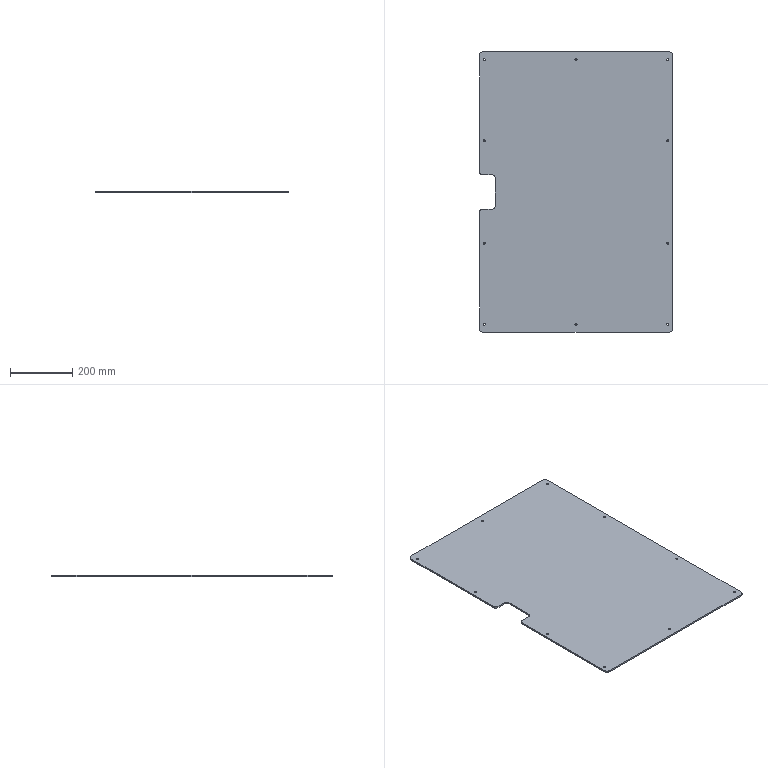Part | STEP file | 11-FG-00911 | 1 solid | 38 faces | box 618 x 900 x 5 mm | volume 2751412 mm3 | cylinder 28 | plane 10 | commonest cylinder face diameters 6.5 x20 20 x8
STEP:
#1=CARTESIAN_POINT('',(-3.25,424.,0.));
#2=VERTEX_POINT('',#1);
#3=CARTESIAN_POINT('',(3.25,424.,0.));
#4=VERTEX_POINT('',#3);
#5=CARTESIAN_POINT('',(0.,424.,0.));
#6=DIRECTION('',(0.,0.,1.));
#7=DIRECTION('',(1.,0.,0.));
#8=AXIS2_PLACEMENT_3D('',#5,#6,#7);
#9=CIRCLE('',#8,3.25);
#10=EDGE_CURVE('',#2,#4,#9,.T.);
#11=ORIENTED_EDGE('',*,*,#10,.F.);
#12=CARTESIAN_POINT('',(-3.25,424.,5.));
#13=VERTEX_POINT('',#12);
#14=CARTESIAN_POINT('',(-3.25,424.,-5.));
#15=DIRECTION('',(0.,0.,1.));
#16=VECTOR('',#15,1000.);
#17=LINE('',#14,#16);
#18=EDGE_CURVE('',#2,#13,#17,.T.);
#19=ORIENTED_EDGE('',*,*,#18,.T.);
#20=CARTESIAN_POINT('',(3.25,424.,5.));
#21=VERTEX_POINT('',#20);
#22=CARTESIAN_POINT('',(0.,424.,5.));
#23=DIRECTION('',(0.,0.,1.));
#24=DIRECTION('',(1.,0.,0.));
#25=AXIS2_PLACEMENT_3D('',#22,#23,#24);
#26=CIRCLE('',#25,3.25);
#27=EDGE_CURVE('',#13,#21,#26,.T.);
#28=ORIENTED_EDGE('',*,*,#27,.T.);
#29=CARTESIAN_POINT('',(3.25,424.,-5.));
#30=DIRECTION('',(0.,0.,1.));
#31=VECTOR('',#30,1000.);
#32=LINE('',#29,#31);
#33=EDGE_CURVE('',#4,#21,#32,.T.);
#34=ORIENTED_EDGE('',*,*,#33,.F.);
#35=EDGE_LOOP('',(#11,#19,#28,#34));
#36=FACE_OUTER_BOUND('',#35,.T.);
#37=CARTESIAN_POINT('',(0.,424.,-5.));
#38=DIRECTION('',(0.,0.,1.));
#39=DIRECTION('',(1.,0.,0.));
#40=AXIS2_PLACEMENT_3D('',#37,#38,#39);
#41=CYLINDRICAL_SURFACE('',#40,3.25);
#42=ADVANCED_FACE('',(#36),#41,.F.);
#43=CARTESIAN_POINT('',(-297.25,424.,0.));
#44=VERTEX_POINT('',#43);
#45=CARTESIAN_POINT('',(-290.75,424.,0.));
#46=VERTEX_POINT('',#45);
#47=CARTESIAN_POINT('',(-294.,424.,0.));
#48=DIRECTION('',(0.,0.,1.));
#49=DIRECTION('',(1.,0.,0.));
#50=AXIS2_PLACEMENT_3D('',#47,#48,#49);
#51=CIRCLE('',#50,3.25);
#52=EDGE_CURVE('',#44,#46,#51,.T.);
#53=ORIENTED_EDGE('',*,*,#52,.F.);
#54=CARTESIAN_POINT('',(-297.25,424.,5.));
#55=VERTEX_POINT('',#54);
#56=CARTESIAN_POINT('',(-297.25,424.,-5.));
#57=DIRECTION('',(0.,0.,1.));
#58=VECTOR('',#57,1000.);
#59=LINE('',#56,#58);
#60=EDGE_CURVE('',#44,#55,#59,.T.);
#61=ORIENTED_EDGE('',*,*,#60,.T.);
#62=CARTESIAN_POINT('',(-290.75,424.,5.));
#63=VERTEX_POINT('',#62);
#64=CARTESIAN_POINT('',(-294.,424.,5.));
#65=DIRECTION('',(0.,0.,1.));
#66=DIRECTION('',(1.,0.,0.));
#67=AXIS2_PLACEMENT_3D('',#64,#65,#66);
#68=CIRCLE('',#67,3.25);
#69=EDGE_CURVE('',#55,#63,#68,.T.);
#70=ORIENTED_EDGE('',*,*,#69,.T.);
#71=CARTESIAN_POINT('',(-290.75,424.,-5.));
#72=DIRECTION('',(0.,0.,1.));
#73=VECTOR('',#72,1000.);
#74=LINE('',#71,#73);
#75=EDGE_CURVE('',#46,#63,#74,.T.);
#76=ORIENTED_EDGE('',*,*,#75,.F.);
#77=EDGE_LOOP('',(#53,#61,#70,#76));
#78=FACE_OUTER_BOUND('',#77,.T.);
#79=CARTESIAN_POINT('',(-294.,424.,-5.));
#80=DIRECTION('',(0.,0.,1.));
#81=DIRECTION('',(1.,0.,0.));
#82=AXIS2_PLACEMENT_3D('',#79,#80,#81);
#83=CYLINDRICAL_SURFACE('',#82,3.25);
#84=ADVANCED_FACE('',(#78),#83,.F.);
#85=CARTESIAN_POINT('',(-297.25,164.,0.));
#86=VERTEX_POINT('',#85);
#87=CARTESIAN_POINT('',(-290.75,164.,0.));
#88=VERTEX_POINT('',#87);
#89=CARTESIAN_POINT('',(-294.,164.,0.));
#90=DIRECTION('',(0.,0.,1.));
#91=DIRECTION('',(1.,0.,0.));
#92=AXIS2_PLACEMENT_3D('',#89,#90,#91);
#93=CIRCLE('',#92,3.25);
#94=EDGE_CURVE('',#86,#88,#93,.T.);
#95=ORIENTED_EDGE('',*,*,#94,.F.);
#96=CARTESIAN_POINT('',(-297.25,164.,5.));
#97=VERTEX_POINT('',#96);
#98=CARTESIAN_POINT('',(-297.25,164.,-5.));
#99=DIRECTION('',(0.,0.,1.));
#100=VECTOR('',#99,1000.);
#101=LINE('',#98,#100);
#102=EDGE_CURVE('',#86,#97,#101,.T.);
#103=ORIENTED_EDGE('',*,*,#102,.T.);
#104=CARTESIAN_POINT('',(-290.75,164.,5.));
#105=VERTEX_POINT('',#104);
#106=CARTESIAN_POINT('',(-294.,164.,5.));
#107=DIRECTION('',(0.,0.,1.));
#108=DIRECTION('',(1.,0.,0.));
#109=AXIS2_PLACEMENT_3D('',#106,#107,#108);
#110=CIRCLE('',#109,3.25);
#111=EDGE_CURVE('',#97,#105,#110,.T.);
#112=ORIENTED_EDGE('',*,*,#111,.T.);
#113=CARTESIAN_POINT('',(-290.75,164.,-5.));
#114=DIRECTION('',(0.,0.,1.));
#115=VECTOR('',#114,1000.);
#116=LINE('',#113,#115);
#117=EDGE_CURVE('',#88,#105,#116,.T.);
#118=ORIENTED_EDGE('',*,*,#117,.F.);
#119=EDGE_LOOP('',(#95,#103,#112,#118));
#120=FACE_OUTER_BOUND('',#119,.T.);
#121=CARTESIAN_POINT('',(-294.,164.,-5.));
#122=DIRECTION('',(0.,0.,1.));
#123=DIRECTION('',(1.,0.,0.));
#124=AXIS2_PLACEMENT_3D('',#121,#122,#123);
#125=CYLINDRICAL_SURFACE('',#124,3.25);
#126=ADVANCED_FACE('',(#120),#125,.F.);
#127=CARTESIAN_POINT('',(-297.25,-164.,0.));
#128=VERTEX_POINT('',#127);
#129=CARTESIAN_POINT('',(-290.75,-164.,0.));
#130=VERTEX_POINT('',#129);
#131=CARTESIAN_POINT('',(-294.,-164.,0.));
#132=DIRECTION('',(0.,0.,1.));
#133=DIRECTION('',(1.,0.,0.));
#134=AXIS2_PLACEMENT_3D('',#131,#132,#133);
#135=CIRCLE('',#134,3.25);
#136=EDGE_CURVE('',#128,#130,#135,.T.);
#137=ORIENTED_EDGE('',*,*,#136,.F.);
#138=CARTESIAN_POINT('',(-297.25,-164.,5.));
#139=VERTEX_POINT('',#138);
#140=CARTESIAN_POINT('',(-297.25,-164.,-5.));
#141=DIRECTION('',(0.,0.,1.));
#142=VECTOR('',#141,1000.);
#143=LINE('',#140,#142);
#144=EDGE_CURVE('',#128,#139,#143,.T.);
#145=ORIENTED_EDGE('',*,*,#144,.T.);
#146=CARTESIAN_POINT('',(-290.75,-164.,5.));
#147=VERTEX_POINT('',#146);
#148=CARTESIAN_POINT('',(-294.,-164.,5.));
#149=DIRECTION('',(0.,0.,1.));
#150=DIRECTION('',(1.,0.,0.));
#151=AXIS2_PLACEMENT_3D('',#148,#149,#150);
#152=CIRCLE('',#151,3.25);
#153=EDGE_CURVE('',#139,#147,#152,.T.);
#154=ORIENTED_EDGE('',*,*,#153,.T.);
#155=CARTESIAN_POINT('',(-290.75,-164.,-5.));
#156=DIRECTION('',(0.,0.,1.));
#157=VECTOR('',#156,1000.);
#158=LINE('',#155,#157);
#159=EDGE_CURVE('',#130,#147,#158,.T.);
#160=ORIENTED_EDGE('',*,*,#159,.F.);
#161=EDGE_LOOP('',(#137,#145,#154,#160));
#162=FACE_OUTER_BOUND('',#161,.T.);
#163=CARTESIAN_POINT('',(-294.,-164.,-5.));
#164=DIRECTION('',(0.,0.,1.));
#165=DIRECTION('',(1.,0.,0.));
#166=AXIS2_PLACEMENT_3D('',#163,#164,#165);
#167=CYLINDRICAL_SURFACE('',#166,3.25);
#168=ADVANCED_FACE('',(#162),#167,.F.);
#169=CARTESIAN_POINT('',(-297.25,-424.,0.));
#170=VERTEX_POINT('',#169);
#171=CARTESIAN_POINT('',(-290.75,-424.,0.));
#172=VERTEX_POINT('',#171);
#173=CARTESIAN_POINT('',(-294.,-424.,0.));
#174=DIRECTION('',(0.,0.,1.));
#175=DIRECTION('',(1.,0.,0.));
#176=AXIS2_PLACEMENT_3D('',#173,#174,#175);
#177=CIRCLE('',#176,3.25);
#178=EDGE_CURVE('',#170,#172,#177,.T.);
#179=ORIENTED_EDGE('',*,*,#178,.F.);
#180=CARTESIAN_POINT('',(-297.25,-424.,5.));
#181=VERTEX_POINT('',#180);
#182=CARTESIAN_POINT('',(-297.25,-424.,-5.));
#183=DIRECTION('',(0.,0.,1.));
#184=VECTOR('',#183,1000.);
#185=LINE('',#182,#184);
#186=EDGE_CURVE('',#170,#181,#185,.T.);
#187=ORIENTED_EDGE('',*,*,#186,.T.);
#188=CARTESIAN_POINT('',(-290.75,-424.,5.));
#189=VERTEX_POINT('',#188);
#190=CARTESIAN_POINT('',(-294.,-424.,5.));
#191=DIRECTION('',(0.,0.,1.));
#192=DIRECTION('',(1.,0.,0.));
#193=AXIS2_PLACEMENT_3D('',#190,#191,#192);
#194=CIRCLE('',#193,3.25);
#195=EDGE_CURVE('',#181,#189,#194,.T.);
#196=ORIENTED_EDGE('',*,*,#195,.T.);
#197=CARTESIAN_POINT('',(-290.75,-424.,-5.));
#198=DIRECTION('',(0.,0.,1.));
#199=VECTOR('',#198,1000.);
#200=LINE('',#197,#199);
#201=EDGE_CURVE('',#172,#189,#200,.T.);
#202=ORIENTED_EDGE('',*,*,#201,.F.);
#203=EDGE_LOOP('',(#179,#187,#196,#202));
#204=FACE_OUTER_BOUND('',#203,.T.);
#205=CARTESIAN_POINT('',(-294.,-424.,-5.));
#206=DIRECTION('',(0.,0.,1.));
#207=DIRECTION('',(1.,0.,0.));
#208=AXIS2_PLACEMENT_3D('',#205,#206,#207);
#209=CYLINDRICAL_SURFACE('',#208,3.25);
#210=ADVANCED_FACE('',(#204),#209,.F.);
#211=CARTESIAN_POINT('',(-3.25,-424.,0.));
#212=VERTEX_POINT('',#211);
#213=CARTESIAN_POINT('',(3.25,-424.,0.));
#214=VERTEX_POINT('',#213);
#215=CARTESIAN_POINT('',(0.,-424.,0.));
#216=DIRECTION('',(0.,0.,1.));
#217=DIRECTION('',(1.,0.,0.));
#218=AXIS2_PLACEMENT_3D('',#215,#216,#217);
#219=CIRCLE('',#218,3.25);
#220=EDGE_CURVE('',#212,#214,#219,.T.);
#221=ORIENTED_EDGE('',*,*,#220,.F.);
#222=CARTESIAN_POINT('',(-3.25,-424.,5.));
#223=VERTEX_POINT('',#222);
#224=CARTESIAN_POINT('',(-3.25,-424.,-5.));
#225=DIRECTION('',(0.,0.,1.));
#226=VECTOR('',#225,1000.);
#227=LINE('',#224,#226);
#228=EDGE_CURVE('',#212,#223,#227,.T.);
#229=ORIENTED_EDGE('',*,*,#228,.T.);
#230=CARTESIAN_POINT('',(3.25,-424.,5.));
#231=VERTEX_POINT('',#230);
#232=CARTESIAN_POINT('',(0.,-424.,5.));
#233=DIRECTION('',(0.,0.,1.));
#234=DIRECTION('',(1.,0.,0.));
#235=AXIS2_PLACEMENT_3D('',#232,#233,#234);
#236=CIRCLE('',#235,3.25);
#237=EDGE_CURVE('',#223,#231,#236,.T.);
#238=ORIENTED_EDGE('',*,*,#237,.T.);
#239=CARTESIAN_POINT('',(3.25,-424.,-5.));
#240=DIRECTION('',(0.,0.,1.));
#241=VECTOR('',#240,1000.);
#242=LINE('',#239,#241);
#243=EDGE_CURVE('',#214,#231,#242,.T.);
#244=ORIENTED_EDGE('',*,*,#243,.F.);
#245=EDGE_LOOP('',(#221,#229,#238,#244));
#246=FACE_OUTER_BOUND('',#245,.T.);
#247=CARTESIAN_POINT('',(0.,-424.,-5.));
#248=DIRECTION('',(0.,0.,1.));
#249=DIRECTION('',(1.,0.,0.));
#250=AXIS2_PLACEMENT_3D('',#247,#248,#249);
#251=CYLINDRICAL_SURFACE('',#250,3.25);
#252=ADVANCED_FACE('',(#246),#251,.F.);
#253=CARTESIAN_POINT('',(290.75,-424.,0.));
#254=VERTEX_POINT('',#253);
#255=CARTESIAN_POINT('',(297.25,-424.,0.));
#256=VERTEX_POINT('',#255);
#257=CARTESIAN_POINT('',(294.,-424.,0.));
#258=DIRECTION('',(0.,0.,1.));
#259=DIRECTION('',(1.,0.,0.));
#260=AXIS2_PLACEMENT_3D('',#257,#258,#259);
#261=CIRCLE('',#260,3.25);
#262=EDGE_CURVE('',#254,#256,#261,.T.);
#263=ORIENTED_EDGE('',*,*,#262,.F.);
#264=CARTESIAN_POINT('',(290.75,-424.,5.));
#265=VERTEX_POINT('',#264);
#266=CARTESIAN_POINT('',(290.75,-424.,-5.));
#267=DIRECTION('',(0.,0.,1.));
#268=VECTOR('',#267,1000.);
#269=LINE('',#266,#268);
#270=EDGE_CURVE('',#254,#265,#269,.T.);
#271=ORIENTED_EDGE('',*,*,#270,.T.);
#272=CARTESIAN_POINT('',(297.25,-424.,5.));
#273=VERTEX_POINT('',#272);
#274=CARTESIAN_POINT('',(294.,-424.,5.));
#275=DIRECTION('',(0.,0.,1.));
#276=DIRECTION('',(1.,0.,0.));
#277=AXIS2_PLACEMENT_3D('',#274,#275,#276);
#278=CIRCLE('',#277,3.25);
#279=EDGE_CURVE('',#265,#273,#278,.T.);
#280=ORIENTED_EDGE('',*,*,#279,.T.);
#281=CARTESIAN_POINT('',(297.25,-424.,-5.));
#282=DIRECTION('',(0.,0.,1.));
#283=VECTOR('',#282,1000.);
#284=LINE('',#281,#283);
#285=EDGE_CURVE('',#256,#273,#284,.T.);
#286=ORIENTED_EDGE('',*,*,#285,.F.);
#287=EDGE_LOOP('',(#263,#271,#280,#286));
#288=FACE_OUTER_BOUND('',#287,.T.);
#289=CARTESIAN_POINT('',(294.,-424.,-5.));
#290=DIRECTION('',(0.,0.,1.));
#291=DIRECTION('',(1.,0.,0.));
#292=AXIS2_PLACEMENT_3D('',#289,#290,#291);
#293=CYLINDRICAL_SURFACE('',#292,3.25);
#294=ADVANCED_FACE('',(#288),#293,.F.);
#295=CARTESIAN_POINT('',(290.75,-164.,0.));
#296=VERTEX_POINT('',#295);
#297=CARTESIAN_POINT('',(297.25,-164.,0.));
#298=VERTEX_POINT('',#297);
#299=CARTESIAN_POINT('',(294.,-164.,0.));
#300=DIRECTION('',(0.,0.,1.));
#301=DIRECTION('',(1.,0.,0.));
#302=AXIS2_PLACEMENT_3D('',#299,#300,#301);
#303=CIRCLE('',#302,3.25);
#304=EDGE_CURVE('',#296,#298,#303,.T.);
#305=ORIENTED_EDGE('',*,*,#304,.F.);
#306=CARTESIAN_POINT('',(290.75,-164.,5.));
#307=VERTEX_POINT('',#306);
#308=CARTESIAN_POINT('',(290.75,-164.,-5.));
#309=DIRECTION('',(0.,0.,1.));
#310=VECTOR('',#309,1000.);
#311=LINE('',#308,#310);
#312=EDGE_CURVE('',#296,#307,#311,.T.);
#313=ORIENTED_EDGE('',*,*,#312,.T.);
#314=CARTESIAN_POINT('',(297.25,-164.,5.));
#315=VERTEX_POINT('',#314);
#316=CARTESIAN_POINT('',(294.,-164.,5.));
#317=DIRECTION('',(0.,0.,1.));
#318=DIRECTION('',(1.,0.,0.));
#319=AXIS2_PLACEMENT_3D('',#316,#317,#318);
#320=CIRCLE('',#319,3.25);
#321=EDGE_CURVE('',#307,#315,#320,.T.);
#322=ORIENTED_EDGE('',*,*,#321,.T.);
#323=CARTESIAN_POINT('',(297.25,-164.,-5.));
#324=DIRECTION('',(0.,0.,1.));
#325=VECTOR('',#324,1000.);
#326=LINE('',#323,#325);
#327=EDGE_CURVE('',#298,#315,#326,.T.);
#328=ORIENTED_EDGE('',*,*,#327,.F.);
#329=EDGE_LOOP('',(#305,#313,#322,#328));
#330=FACE_OUTER_BOUND('',#329,.T.);
#331=CARTESIAN_POINT('',(294.,-164.,-5.));
#332=DIRECTION('',(0.,0.,1.));
#333=DIRECTION('',(1.,0.,0.));
#334=AXIS2_PLACEMENT_3D('',#331,#332,#333);
#335=CYLINDRICAL_SURFACE('',#334,3.25);
#336=ADVANCED_FACE('',(#330),#335,.F.);
#337=CARTESIAN_POINT('',(290.75,164.,0.));
#338=VERTEX_POINT('',#337);
#339=CARTESIAN_POINT('',(297.25,164.,0.));
#340=VERTEX_POINT('',#339);
#341=CARTESIAN_POINT('',(294.,164.,0.));
#342=DIRECTION('',(0.,0.,1.));
#343=DIRECTION('',(1.,0.,0.));
#344=AXIS2_PLACEMENT_3D('',#341,#342,#343);
#345=CIRCLE('',#344,3.25);
#346=EDGE_CURVE('',#338,#340,#345,.T.);
#347=ORIENTED_EDGE('',*,*,#346,.F.);
#348=CARTESIAN_POINT('',(290.75,164.,5.));
#349=VERTEX_POINT('',#348);
#350=CARTESIAN_POINT('',(290.75,164.,-5.));
#351=DIRECTION('',(0.,0.,1.));
#352=VECTOR('',#351,1000.);
#353=LINE('',#350,#352);
#354=EDGE_CURVE('',#338,#349,#353,.T.);
#355=ORIENTED_EDGE('',*,*,#354,.T.);
#356=CARTESIAN_POINT('',(297.25,164.,5.));
#357=VERTEX_POINT('',#356);
#358=CARTESIAN_POINT('',(294.,164.,5.));
#359=DIRECTION('',(0.,0.,1.));
#360=DIRECTION('',(1.,0.,0.));
#361=AXIS2_PLACEMENT_3D('',#358,#359,#360);
#362=CIRCLE('',#361,3.25);
#363=EDGE_CURVE('',#349,#357,#362,.T.);
#364=ORIENTED_EDGE('',*,*,#363,.T.);
#365=CARTESIAN_POINT('',(297.25,164.,-5.));
#366=DIRECTION('',(0.,0.,1.));
#367=VECTOR('',#366,1000.);
#368=LINE('',#365,#367);
#369=EDGE_CURVE('',#340,#357,#368,.T.);
#370=ORIENTED_EDGE('',*,*,#369,.F.);
#371=EDGE_LOOP('',(#347,#355,#364,#370));
#372=FACE_OUTER_BOUND('',#371,.T.);
#373=CARTESIAN_POINT('',(294.,164.,-5.));
#374=DIRECTION('',(0.,0.,1.));
#375=DIRECTION('',(1.,0.,0.));
#376=AXIS2_PLACEMENT_3D('',#373,#374,#375);
#377=CYLINDRICAL_SURFACE('',#376,3.25);
#378=ADVANCED_FACE('',(#372),#377,.F.);
#379=CARTESIAN_POINT('',(290.75,424.,0.));
#380=VERTEX_POINT('',#379);
#381=CARTESIAN_POINT('',(297.25,424.,0.));
#382=VERTEX_POINT('',#381);
#383=CARTESIAN_POINT('',(294.,424.,0.));
#384=DIRECTION('',(0.,0.,1.));
#385=DIRECTION('',(1.,0.,0.));
#386=AXIS2_PLACEMENT_3D('',#383,#384,#385);
#387=CIRCLE('',#386,3.25);
#388=EDGE_CURVE('',#380,#382,#387,.T.);
#389=ORIENTED_EDGE('',*,*,#388,.F.);
#390=CARTESIAN_POINT('',(290.75,424.,5.));
#391=VERTEX_POINT('',#390);
#392=CARTESIAN_POINT('',(290.75,424.,-5.));
#393=DIRECTION('',(0.,0.,1.));
#394=VECTOR('',#393,1000.);
#395=LINE('',#392,#394);
#396=EDGE_CURVE('',#380,#391,#395,.T.);
#397=ORIENTED_EDGE('',*,*,#396,.T.);
#398=CARTESIAN_POINT('',(297.25,424.,5.));
#399=VERTEX_POINT('',#398);
#400=CARTESIAN_POINT('',(294.,424.,5.));
#401=DIRECTION('',(0.,0.,1.));
#402=DIRECTION('',(1.,0.,0.));
#403=AXIS2_PLACEMENT_3D('',#400,#401,#402);
#404=CIRCLE('',#403,3.25);
#405=EDGE_CURVE('',#391,#399,#404,.T.);
#406=ORIENTED_EDGE('',*,*,#405,.T.);
#407=CARTESIAN_POINT('',(297.25,424.,-5.));
#408=DIRECTION('',(0.,0.,1.));
#409=VECTOR('',#408,1000.);
#410=LINE('',#407,#409);
#411=EDGE_CURVE('',#382,#399,#410,.T.);
#412=ORIENTED_EDGE('',*,*,#411,.F.);
#413=EDGE_LOOP('',(#389,#397,#406,#412));
#414=FACE_OUTER_BOUND('',#413,.T.);
#415=CARTESIAN_POINT('',(294.,424.,-5.));
#416=DIRECTION('',(0.,0.,1.));
#417=DIRECTION('',(1.,0.,0.));
#418=AXIS2_PLACEMENT_3D('',#415,#416,#417);
#419=CYLINDRICAL_SURFACE('',#418,3.25);
#420=ADVANCED_FACE('',(#414),#419,.F.);
#421=CARTESIAN_POINT('',(-309.,440.,0.));
#422=VERTEX_POINT('',#421);
#423=CARTESIAN_POINT('',(-309.,65.,0.));
#424=VERTEX_POINT('',#423);
#425=CARTESIAN_POINT('',(-309.,450.,0.));
#426=DIRECTION('',(0.,-1.,0.));
#427=VECTOR('',#426,1000.);
#428=LINE('',#425,#427);
#429=EDGE_CURVE('',#422,#424,#428,.T.);
#430=ORIENTED_EDGE('',*,*,#429,.T.);
#431=CARTESIAN_POINT('',(-309.,65.,5.));
#432=VERTEX_POINT('',#431);
#433=CARTESIAN_POINT('',(-309.,65.,5.));
#434=DIRECTION('',(0.,0.,1.));
#435=VECTOR('',#434,1000.);
#436=LINE('',#433,#435);
#437=EDGE_CURVE('',#424,#432,#436,.T.);
#438=ORIENTED_EDGE('',*,*,#437,.T.);
#439=CARTESIAN_POINT('',(-309.,440.,5.));
#440=VERTEX_POINT('',#439);
#441=CARTESIAN_POINT('',(-309.,450.,5.));
#442=DIRECTION('',(0.,-1.,0.));
#443=VECTOR('',#442,1000.);
#444=LINE('',#441,#443);
#445=EDGE_CURVE('',#440,#432,#444,.T.);
#446=ORIENTED_EDGE('',*,*,#445,.F.);
#447=CARTESIAN_POINT('',(-309.,440.,5.));
#448=DIRECTION('',(0.,0.,-1.));
#449=VECTOR('',#448,1000.);
#450=LINE('',#447,#449);
#451=EDGE_CURVE('',#440,#422,#450,.T.);
#452=ORIENTED_EDGE('',*,*,#451,.T.);
#453=EDGE_LOOP('',(#430,#438,#446,#452));
#454=FACE_OUTER_BOUND('',#453,.T.);
#455=CARTESIAN_POINT('',(-309.,450.,5.));
#456=DIRECTION('',(1.,0.,0.));
#457=DIRECTION('',(0.,1.,0.));
#458=AXIS2_PLACEMENT_3D('',#455,#456,#457);
#459=PLANE('',#458);
#460=ADVANCED_FACE('',(#454),#459,.F.);
#461=CARTESIAN_POINT('',(309.,-440.,5.));
#462=VERTEX_POINT('',#461);
#463=CARTESIAN_POINT('',(309.,440.,5.));
#464=VERTEX_POINT('',#463);
#465=CARTESIAN_POINT('',(309.,450.,5.));
#466=DIRECTION('',(0.,1.,0.));
#467=VECTOR('',#466,1000.);
#468=LINE('',#465,#467);
#469=EDGE_CURVE('',#462,#464,#468,.T.);
#470=ORIENTED_EDGE('',*,*,#469,.F.);
#471=CARTESIAN_POINT('',(309.,-440.,0.));
#472=VERTEX_POINT('',#471);
#473=CARTESIAN_POINT('',(309.,-440.,5.));
#474=DIRECTION('',(0.,0.,-1.));
#475=VECTOR('',#474,1000.);
#476=LINE('',#473,#475);
#477=EDGE_CURVE('',#462,#472,#476,.T.);
#478=ORIENTED_EDGE('',*,*,#477,.T.);
#479=CARTESIAN_POINT('',(309.,440.,0.));
#480=VERTEX_POINT('',#479);
#481=CARTESIAN_POINT('',(309.,450.,0.));
#482=DIRECTION('',(0.,1.,0.));
#483=VECTOR('',#482,1000.);
#484=LINE('',#481,#483);
#485=EDGE_CURVE('',#472,#480,#484,.T.);
#486=ORIENTED_EDGE('',*,*,#485,.T.);
#487=CARTESIAN_POINT('',(309.,440.,5.));
#488=DIRECTION('',(0.,0.,1.));
#489=VECTOR('',#488,1000.);
#490=LINE('',#487,#489);
#491=EDGE_CURVE('',#480,#464,#490,.T.);
#492=ORIENTED_EDGE('',*,*,#491,.T.);
#493=EDGE_LOOP('',(#470,#478,#486,#492));
#494=FACE_OUTER_BOUND('',#493,.T.);
#495=CARTESIAN_POINT('',(309.,450.,5.));
#496=DIRECTION('',(-1.,0.,0.));
#497=DIRECTION('',(0.,-1.,0.));
#498=AXIS2_PLACEMENT_3D('',#495,#496,#497);
#499=PLANE('',#498);
#500=ADVANCED_FACE('',(#494),#499,.F.);
#501=CARTESIAN_POINT('',(299.,450.,5.));
#502=VERTEX_POINT('',#501);
#503=CARTESIAN_POINT('',(-299.,450.,5.));
#504=VERTEX_POINT('',#503);
#505=CARTESIAN_POINT('',(-309.,450.,5.));
#506=DIRECTION('',(-1.,0.,0.));
#507=VECTOR('',#506,1000.);
#508=LINE('',#505,#507);
#509=EDGE_CURVE('',#502,#504,#508,.T.);
#510=ORIENTED_EDGE('',*,*,#509,.F.);
#511=CARTESIAN_POINT('',(299.,450.,0.));
#512=VERTEX_POINT('',#511);
#513=CARTESIAN_POINT('',(299.,450.,5.));
#514=DIRECTION('',(0.,0.,-1.));
#515=VECTOR('',#514,1000.);
#516=LINE('',#513,#515);
#517=EDGE_CURVE('',#502,#512,#516,.T.);
#518=ORIENTED_EDGE('',*,*,#517,.T.);
#519=CARTESIAN_POINT('',(-299.,450.,0.));
#520=VERTEX_POINT('',#519);
#521=CARTESIAN_POINT('',(-309.,450.,0.));
#522=DIRECTION('',(-1.,0.,0.));
#523=VECTOR('',#522,1000.);
#524=LINE('',#521,#523);
#525=EDGE_CURVE('',#512,#520,#524,.T.);
#526=ORIENTED_EDGE('',*,*,#525,.T.);
#527=CARTESIAN_POINT('',(-299.,450.,5.));
#528=DIRECTION('',(0.,0.,1.));
#529=VECTOR('',#528,1000.);
#530=LINE('',#527,#529);
#531=EDGE_CURVE('',#520,#504,#530,.T.);
#532=ORIENTED_EDGE('',*,*,#531,.T.);
#533=EDGE_LOOP('',(#510,#518,#526,#532));
#534=FACE_OUTER_BOUND('',#533,.T.);
#535=CARTESIAN_POINT('',(-309.,450.,5.));
#536=DIRECTION('',(0.,-1.,0.));
#537=DIRECTION('',(0.,0.,-1.));
#538=AXIS2_PLACEMENT_3D('',#535,#536,#537);
#539=PLANE('',#538);
#540=ADVANCED_FACE('',(#534),#539,.F.);
#541=CARTESIAN_POINT('',(-309.,-65.,5.));
#542=VERTEX_POINT('',#541);
#543=CARTESIAN_POINT('',(-309.,-440.,5.));
#544=VERTEX_POINT('',#543);
#545=CARTESIAN_POINT('',(-309.,450.,5.));
#546=DIRECTION('',(0.,-1.,0.));
#547=VECTOR('',#546,1000.);
#548=LINE('',#545,#547);
#549=EDGE_CURVE('',#542,#544,#548,.T.);
#550=ORIENTED_EDGE('',*,*,#549,.F.);
#551=CARTESIAN_POINT('',(-309.,-65.,0.));
#552=VERTEX_POINT('',#551);
#553=CARTESIAN_POINT('',(-309.,-65.,5.));
#554=DIRECTION('',(0.,0.,-1.));
#555=VECTOR('',#554,1000.);
#556=LINE('',#553,#555);
#557=EDGE_CURVE('',#542,#552,#556,.T.);
#558=ORIENTED_EDGE('',*,*,#557,.T.);
#559=CARTESIAN_POINT('',(-309.,-440.,0.));
#560=VERTEX_POINT('',#559);
#561=CARTESIAN_POINT('',(-309.,450.,0.));
#562=DIRECTION('',(0.,-1.,0.));
#563=VECTOR('',#562,1000.);
#564=LINE('',#561,#563);
#565=EDGE_CURVE('',#552,#560,#564,.T.);
#566=ORIENTED_EDGE('',*,*,#565,.T.);
#567=CARTESIAN_POINT('',(-309.,-440.,5.));
#568=DIRECTION('',(0.,0.,1.));
#569=VECTOR('',#568,1000.);
#570=LINE('',#567,#569);
#571=EDGE_CURVE('',#560,#544,#570,.T.);
#572=ORIENTED_EDGE('',*,*,#571,.T.);
#573=EDGE_LOOP('',(#550,#558,#566,#572));
#574=FACE_OUTER_BOUND('',#573,.T.);
#575=CARTESIAN_POINT('',(-309.,450.,5.));
#576=DIRECTION('',(1.,0.,0.));
#577=DIRECTION('',(0.,1.,0.));
#578=AXIS2_PLACEMENT_3D('',#575,#576,#577);
#579=PLANE('',#578);
#580=ADVANCED_FACE('',(#574),#579,.F.);
#581=CARTESIAN_POINT('',(-299.,-450.,5.));
#582=VERTEX_POINT('',#581);
#583=CARTESIAN_POINT('',(299.,-450.,5.));
#584=VERTEX_POINT('',#583);
#585=CARTESIAN_POINT('',(-309.,-450.,5.));
#586=DIRECTION('',(1.,0.,0.));
#587=VECTOR('',#586,1000.);
#588=LINE('',#585,#587);
#589=EDGE_CURVE('',#582,#584,#588,.T.);
#590=ORIENTED_EDGE('',*,*,#589,.F.);
#591=CARTESIAN_POINT('',(-299.,-450.,0.));
#592=VERTEX_POINT('',#591);
#593=CARTESIAN_POINT('',(-299.,-450.,5.));
#594=DIRECTION('',(0.,0.,-1.));
#595=VECTOR('',#594,1000.);
#596=LINE('',#593,#595);
#597=EDGE_CURVE('',#582,#592,#596,.T.);
#598=ORIENTED_EDGE('',*,*,#597,.T.);
#599=CARTESIAN_POINT('',(299.,-450.,0.));
#600=VERTEX_POINT('',#599);
#601=CARTESIAN_POINT('',(-309.,-450.,0.));
#602=DIRECTION('',(1.,0.,0.));
#603=VECTOR('',#602,1000.);
#604=LINE('',#601,#603);
#605=EDGE_CURVE('',#592,#600,#604,.T.);
#606=ORIENTED_EDGE('',*,*,#605,.T.);
#607=CARTESIAN_POINT('',(299.,-450.,5.));
#608=DIRECTION('',(0.,0.,1.));
#609=VECTOR('',#608,1000.);
#610=LINE('',#607,#609);
#611=EDGE_CURVE('',#600,#584,#610,.T.);
#612=ORIENTED_EDGE('',*,*,#611,.T.);
#613=EDGE_LOOP('',(#590,#598,#606,#612));
#614=FACE_OUTER_BOUND('',#613,.T.);
#615=CARTESIAN_POINT('',(-309.,-450.,5.));
#616=DIRECTION('',(0.,1.,0.));
#617=DIRECTION('',(0.,0.,1.));
#618=AXIS2_PLACEMENT_3D('',#615,#616,#617);
#619=PLANE('',#618);
#620=ADVANCED_FACE('',(#614),#619,.F.);
#621=CARTESIAN_POINT('',(0.,424.,5.));
#622=DIRECTION('',(0.,0.,1.));
#623=DIRECTION('',(1.,0.,0.));
#624=AXIS2_PLACEMENT_3D('',#621,#622,#623);
#625=CIRCLE('',#624,3.25);
#626=EDGE_CURVE('',#21,#13,#625,.T.);
#627=ORIENTED_EDGE('',*,*,#626,.F.);
#628=ORIENTED_EDGE('',*,*,#27,.F.);
#629=EDGE_LOOP('',(#627,#628));
#630=FACE_BOUND('',#629,.T.);
#631=CARTESIAN_POINT('',(-294.,424.,5.));
#632=DIRECTION('',(0.,0.,1.));
#633=DIRECTION('',(1.,0.,0.));
#634=AXIS2_PLACEMENT_3D('',#631,#632,#633);
#635=CIRCLE('',#634,3.25);
#636=EDGE_CURVE('',#63,#55,#635,.T.);
#637=ORIENTED_EDGE('',*,*,#636,.F.);
#638=ORIENTED_EDGE('',*,*,#69,.F.);
#639=EDGE_LOOP('',(#637,#638));
#640=FACE_BOUND('',#639,.T.);
#641=CARTESIAN_POINT('',(-294.,164.,5.));
#642=DIRECTION('',(0.,0.,1.));
#643=DIRECTION('',(1.,0.,0.));
#644=AXIS2_PLACEMENT_3D('',#641,#642,#643);
#645=CIRCLE('',#644,3.25);
#646=EDGE_CURVE('',#105,#97,#645,.T.);
#647=ORIENTED_EDGE('',*,*,#646,.F.);
#648=ORIENTED_EDGE('',*,*,#111,.F.);
#649=EDGE_LOOP('',(#647,#648));
#650=FACE_BOUND('',#649,.T.);
#651=CARTESIAN_POINT('',(-294.,-164.,5.));
#652=DIRECTION('',(0.,0.,1.));
#653=DIRECTION('',(1.,0.,0.));
#654=AXIS2_PLACEMENT_3D('',#651,#652,#653);
#655=CIRCLE('',#654,3.25);
#656=EDGE_CURVE('',#147,#139,#655,.T.);
#657=ORIENTED_EDGE('',*,*,#656,.F.);
#658=ORIENTED_EDGE('',*,*,#153,.F.);
#659=EDGE_LOOP('',(#657,#658));
#660=FACE_BOUND('',#659,.T.);
#661=CARTESIAN_POINT('',(-294.,-424.,5.));
#662=DIRECTION('',(0.,0.,1.));
#663=DIRECTION('',(1.,0.,0.));
#664=AXIS2_PLACEMENT_3D('',#661,#662,#663);
#665=CIRCLE('',#664,3.25);
#666=EDGE_CURVE('',#189,#181,#665,.T.);
#667=ORIENTED_EDGE('',*,*,#666,.F.);
#668=ORIENTED_EDGE('',*,*,#195,.F.);
#669=EDGE_LOOP('',(#667,#668));
#670=FACE_BOUND('',#669,.T.);
#671=CARTESIAN_POINT('',(0.,-424.,5.));
#672=DIRECTION('',(0.,0.,1.));
#673=DIRECTION('',(1.,0.,0.));
#674=AXIS2_PLACEMENT_3D('',#671,#672,#673);
#675=CIRCLE('',#674,3.25);
#676=EDGE_CURVE('',#231,#223,#675,.T.);
#677=ORIENTED_EDGE('',*,*,#676,.F.);
#678=ORIENTED_EDGE('',*,*,#237,.F.);
#679=EDGE_LOOP('',(#677,#678));
#680=FACE_BOUND('',#679,.T.);
#681=CARTESIAN_POINT('',(294.,-424.,5.));
#682=DIRECTION('',(0.,0.,1.));
#683=DIRECTION('',(1.,0.,0.));
#684=AXIS2_PLACEMENT_3D('',#681,#682,#683);
#685=CIRCLE('',#684,3.25);
#686=EDGE_CURVE('',#273,#265,#685,.T.);
#687=ORIENTED_EDGE('',*,*,#686,.F.);
#688=ORIENTED_EDGE('',*,*,#279,.F.);
#689=EDGE_LOOP('',(#687,#688));
#690=FACE_BOUND('',#689,.T.);
#691=CARTESIAN_POINT('',(294.,-164.,5.));
#692=DIRECTION('',(0.,0.,1.));
#693=DIRECTION('',(1.,0.,0.));
#694=AXIS2_PLACEMENT_3D('',#691,#692,#693);
#695=CIRCLE('',#694,3.25);
#696=EDGE_CURVE('',#315,#307,#695,.T.);
#697=ORIENTED_EDGE('',*,*,#696,.F.);
#698=ORIENTED_EDGE('',*,*,#321,.F.);
#699=EDGE_LOOP('',(#697,#698));
#700=FACE_BOUND('',#699,.T.);
#701=CARTESIAN_POINT('',(294.,164.,5.));
#702=DIRECTION('',(0.,0.,1.));
#703=DIRECTION('',(1.,0.,0.));
#704=AXIS2_PLACEMENT_3D('',#701,#702,#703);
#705=CIRCLE('',#704,3.25);
#706=EDGE_CURVE('',#357,#349,#705,.T.);
#707=ORIENTED_EDGE('',*,*,#706,.F.);
#708=ORIENTED_EDGE('',*,*,#363,.F.);
#709=EDGE_LOOP('',(#707,#708));
#710=FACE_BOUND('',#709,.T.);
#711=CARTESIAN_POINT('',(294.,424.,5.));
#712=DIRECTION('',(0.,0.,1.));
#713=DIRECTION('',(1.,0.,0.));
#714=AXIS2_PLACEMENT_3D('',#711,#712,#713);
#715=CIRCLE('',#714,3.25);
#716=EDGE_CURVE('',#399,#391,#715,.T.);
#717=ORIENTED_EDGE('',*,*,#716,.F.);
#718=ORIENTED_EDGE('',*,*,#405,.F.);
#719=EDGE_LOOP('',(#717,#718));
#720=FACE_BOUND('',#719,.T.);
#721=ORIENTED_EDGE('',*,*,#445,.T.);
#722=CARTESIAN_POINT('',(-299.,55.,5.));
#723=VERTEX_POINT('',#722);
#724=CARTESIAN_POINT('',(-299.,65.,5.));
#725=DIRECTION('',(0.,0.,1.));
#726=DIRECTION('',(1.,0.,0.));
#727=AXIS2_PLACEMENT_3D('',#724,#725,#726);
#728=CIRCLE('',#727,10.);
#729=EDGE_CURVE('',#432,#723,#728,.T.);
#730=ORIENTED_EDGE('',*,*,#729,.T.);
#731=CARTESIAN_POINT('',(-269.,55.,5.));
#732=VERTEX_POINT('',#731);
#733=CARTESIAN_POINT('',(-259.,55.,5.));
#734=DIRECTION('',(-1.,0.,0.));
#735=VECTOR('',#734,1000.);
#736=LINE('',#733,#735);
#737=EDGE_CURVE('',#732,#723,#736,.T.);
#738=ORIENTED_EDGE('',*,*,#737,.F.);
#739=CARTESIAN_POINT('',(-259.,45.,5.));
#740=VERTEX_POINT('',#739);
#741=CARTESIAN_POINT('',(-269.,45.,5.));
#742=DIRECTION('',(0.,0.,-1.));
#743=DIRECTION('',(1.,0.,0.));
#744=AXIS2_PLACEMENT_3D('',#741,#742,#743);
#745=CIRCLE('',#744,10.);
#746=EDGE_CURVE('',#732,#740,#745,.T.);
#747=ORIENTED_EDGE('',*,*,#746,.T.);
#748=CARTESIAN_POINT('',(-259.,-45.,5.));
#749=VERTEX_POINT('',#748);
#750=CARTESIAN_POINT('',(-259.,-55.,5.));
#751=DIRECTION('',(0.,1.,0.));
#752=VECTOR('',#751,1000.);
#753=LINE('',#750,#752);
#754=EDGE_CURVE('',#749,#740,#753,.T.);
#755=ORIENTED_EDGE('',*,*,#754,.F.);
#756=CARTESIAN_POINT('',(-269.,-55.,5.));
#757=VERTEX_POINT('',#756);
#758=CARTESIAN_POINT('',(-269.,-45.,5.));
#759=DIRECTION('',(0.,0.,-1.));
#760=DIRECTION('',(1.,0.,0.));
#761=AXIS2_PLACEMENT_3D('',#758,#759,#760);
#762=CIRCLE('',#761,10.);
#763=EDGE_CURVE('',#749,#757,#762,.T.);
#764=ORIENTED_EDGE('',*,*,#763,.T.);
#765=CARTESIAN_POINT('',(-299.,-55.,5.));
#766=VERTEX_POINT('',#765);
#767=CARTESIAN_POINT('',(-259.,-55.,5.));
#768=DIRECTION('',(1.,0.,0.));
#769=VECTOR('',#768,1000.);
#770=LINE('',#767,#769);
#771=EDGE_CURVE('',#766,#757,#770,.T.);
#772=ORIENTED_EDGE('',*,*,#771,.F.);
#773=CARTESIAN_POINT('',(-299.,-65.,5.));
#774=DIRECTION('',(0.,0.,1.));
#775=DIRECTION('',(1.,0.,0.));
#776=AXIS2_PLACEMENT_3D('',#773,#774,#775);
#777=CIRCLE('',#776,10.);
#778=EDGE_CURVE('',#766,#542,#777,.T.);
#779=ORIENTED_EDGE('',*,*,#778,.T.);
#780=ORIENTED_EDGE('',*,*,#549,.T.);
#781=CARTESIAN_POINT('',(-299.,-440.,5.));
#782=DIRECTION('',(0.,0.,1.));
#783=DIRECTION('',(1.,0.,0.));
#784=AXIS2_PLACEMENT_3D('',#781,#782,#783);
#785=CIRCLE('',#784,10.);
#786=EDGE_CURVE('',#544,#582,#785,.T.);
#787=ORIENTED_EDGE('',*,*,#786,.T.);
#788=ORIENTED_EDGE('',*,*,#589,.T.);
#789=CARTESIAN_POINT('',(299.,-440.,5.));
#790=DIRECTION('',(0.,0.,1.));
#791=DIRECTION('',(1.,0.,0.));
#792=AXIS2_PLACEMENT_3D('',#789,#790,#791);
#793=CIRCLE('',#792,10.);
#794=EDGE_CURVE('',#584,#462,#793,.T.);
#795=ORIENTED_EDGE('',*,*,#794,.T.);
#796=ORIENTED_EDGE('',*,*,#469,.T.);
#797=CARTESIAN_POINT('',(299.,440.,5.));
#798=DIRECTION('',(0.,0.,1.));
#799=DIRECTION('',(1.,0.,0.));
#800=AXIS2_PLACEMENT_3D('',#797,#798,#799);
#801=CIRCLE('',#800,10.);
#802=EDGE_CURVE('',#464,#502,#801,.T.);
#803=ORIENTED_EDGE('',*,*,#802,.T.);
#804=ORIENTED_EDGE('',*,*,#509,.T.);
#805=CARTESIAN_POINT('',(-299.,440.,5.));
#806=DIRECTION('',(0.,0.,1.));
#807=DIRECTION('',(1.,0.,0.));
#808=AXIS2_PLACEMENT_3D('',#805,#806,#807);
#809=CIRCLE('',#808,10.);
#810=EDGE_CURVE('',#504,#440,#809,.T.);
#811=ORIENTED_EDGE('',*,*,#810,.T.);
#812=EDGE_LOOP('',(#721,#730,#738,#747,#755,#764,#772,#779,#780,#787,#788,#795,#796,#803,#804,#811));
#813=FACE_OUTER_BOUND('',#812,.T.);
#814=CARTESIAN_POINT('',(0.,0.,5.));
#815=DIRECTION('',(0.,0.,1.));
#816=DIRECTION('',(1.,0.,0.));
#817=AXIS2_PLACEMENT_3D('',#814,#815,#816);
#818=PLANE('',#817);
#819=ADVANCED_FACE('',(#630,#640,#650,#660,#670,#680,#690,#700,#710,#720,#813),#818,.T.);
#820=CARTESIAN_POINT('',(0.,424.,0.));
#821=DIRECTION('',(0.,0.,1.));
#822=DIRECTION('',(1.,0.,0.));
#823=AXIS2_PLACEMENT_3D('',#820,#821,#822);
#824=CIRCLE('',#823,3.25);
#825=EDGE_CURVE('',#4,#2,#824,.T.);
#826=ORIENTED_EDGE('',*,*,#825,.T.);
#827=ORIENTED_EDGE('',*,*,#10,.T.);
#828=EDGE_LOOP('',(#826,#827));
#829=FACE_BOUND('',#828,.T.);
#830=CARTESIAN_POINT('',(-294.,424.,0.));
#831=DIRECTION('',(0.,0.,1.));
#832=DIRECTION('',(1.,0.,0.));
#833=AXIS2_PLACEMENT_3D('',#830,#831,#832);
#834=CIRCLE('',#833,3.25);
#835=EDGE_CURVE('',#46,#44,#834,.T.);
#836=ORIENTED_EDGE('',*,*,#835,.T.);
#837=ORIENTED_EDGE('',*,*,#52,.T.);
#838=EDGE_LOOP('',(#836,#837));
#839=FACE_BOUND('',#838,.T.);
#840=CARTESIAN_POINT('',(-294.,164.,0.));
#841=DIRECTION('',(0.,0.,1.));
#842=DIRECTION('',(1.,0.,0.));
#843=AXIS2_PLACEMENT_3D('',#840,#841,#842);
#844=CIRCLE('',#843,3.25);
#845=EDGE_CURVE('',#88,#86,#844,.T.);
#846=ORIENTED_EDGE('',*,*,#845,.T.);
#847=ORIENTED_EDGE('',*,*,#94,.T.);
#848=EDGE_LOOP('',(#846,#847));
#849=FACE_BOUND('',#848,.T.);
#850=CARTESIAN_POINT('',(-294.,-164.,0.));
#851=DIRECTION('',(0.,0.,1.));
#852=DIRECTION('',(1.,0.,0.));
#853=AXIS2_PLACEMENT_3D('',#850,#851,#852);
#854=CIRCLE('',#853,3.25);
#855=EDGE_CURVE('',#130,#128,#854,.T.);
#856=ORIENTED_EDGE('',*,*,#855,.T.);
#857=ORIENTED_EDGE('',*,*,#136,.T.);
#858=EDGE_LOOP('',(#856,#857));
#859=FACE_BOUND('',#858,.T.);
#860=CARTESIAN_POINT('',(-294.,-424.,0.));
#861=DIRECTION('',(0.,0.,1.));
#862=DIRECTION('',(1.,0.,0.));
#863=AXIS2_PLACEMENT_3D('',#860,#861,#862);
#864=CIRCLE('',#863,3.25);
#865=EDGE_CURVE('',#172,#170,#864,.T.);
#866=ORIENTED_EDGE('',*,*,#865,.T.);
#867=ORIENTED_EDGE('',*,*,#178,.T.);
#868=EDGE_LOOP('',(#866,#867));
#869=FACE_BOUND('',#868,.T.);
#870=CARTESIAN_POINT('',(0.,-424.,0.));
#871=DIRECTION('',(0.,0.,1.));
#872=DIRECTION('',(1.,0.,0.));
#873=AXIS2_PLACEMENT_3D('',#870,#871,#872);
#874=CIRCLE('',#873,3.25);
#875=EDGE_CURVE('',#214,#212,#874,.T.);
#876=ORIENTED_EDGE('',*,*,#875,.T.);
#877=ORIENTED_EDGE('',*,*,#220,.T.);
#878=EDGE_LOOP('',(#876,#877));
#879=FACE_BOUND('',#878,.T.);
#880=CARTESIAN_POINT('',(294.,-424.,0.));
#881=DIRECTION('',(0.,0.,1.));
#882=DIRECTION('',(1.,0.,0.));
#883=AXIS2_PLACEMENT_3D('',#880,#881,#882);
#884=CIRCLE('',#883,3.25);
#885=EDGE_CURVE('',#256,#254,#884,.T.);
#886=ORIENTED_EDGE('',*,*,#885,.T.);
#887=ORIENTED_EDGE('',*,*,#262,.T.);
#888=EDGE_LOOP('',(#886,#887));
#889=FACE_BOUND('',#888,.T.);
#890=CARTESIAN_POINT('',(294.,-164.,0.));
#891=DIRECTION('',(0.,0.,1.));
#892=DIRECTION('',(1.,0.,0.));
#893=AXIS2_PLACEMENT_3D('',#890,#891,#892);
#894=CIRCLE('',#893,3.25);
#895=EDGE_CURVE('',#298,#296,#894,.T.);
#896=ORIENTED_EDGE('',*,*,#895,.T.);
#897=ORIENTED_EDGE('',*,*,#304,.T.);
#898=EDGE_LOOP('',(#896,#897));
#899=FACE_BOUND('',#898,.T.);
#900=CARTESIAN_POINT('',(294.,164.,0.));
#901=DIRECTION('',(0.,0.,1.));
#902=DIRECTION('',(1.,0.,0.));
#903=AXIS2_PLACEMENT_3D('',#900,#901,#902);
#904=CIRCLE('',#903,3.25);
#905=EDGE_CURVE('',#340,#338,#904,.T.);
#906=ORIENTED_EDGE('',*,*,#905,.T.);
#907=ORIENTED_EDGE('',*,*,#346,.T.);
#908=EDGE_LOOP('',(#906,#907));
#909=FACE_BOUND('',#908,.T.);
#910=CARTESIAN_POINT('',(294.,424.,0.));
#911=DIRECTION('',(0.,0.,1.));
#912=DIRECTION('',(1.,0.,0.));
#913=AXIS2_PLACEMENT_3D('',#910,#911,#912);
#914=CIRCLE('',#913,3.25);
#915=EDGE_CURVE('',#382,#380,#914,.T.);
#916=ORIENTED_EDGE('',*,*,#915,.T.);
#917=ORIENTED_EDGE('',*,*,#388,.T.);
#918=EDGE_LOOP('',(#916,#917));
#919=FACE_BOUND('',#918,.T.);
#920=CARTESIAN_POINT('',(-269.,55.,0.));
#921=VERTEX_POINT('',#920);
#922=CARTESIAN_POINT('',(-299.,55.,0.));
#923=VERTEX_POINT('',#922);
#924=CARTESIAN_POINT('',(-259.,55.,0.));
#925=DIRECTION('',(-1.,0.,0.));
#926=VECTOR('',#925,1000.);
#927=LINE('',#924,#926);
#928=EDGE_CURVE('',#921,#923,#927,.T.);
#929=ORIENTED_EDGE('',*,*,#928,.T.);
#930=CARTESIAN_POINT('',(-299.,65.,0.));
#931=DIRECTION('',(0.,0.,-1.));
#932=DIRECTION('',(1.,0.,0.));
#933=AXIS2_PLACEMENT_3D('',#930,#931,#932);
#934=CIRCLE('',#933,10.);
#935=EDGE_CURVE('',#923,#424,#934,.T.);
#936=ORIENTED_EDGE('',*,*,#935,.T.);
#937=ORIENTED_EDGE('',*,*,#429,.F.);
#938=CARTESIAN_POINT('',(-299.,440.,0.));
#939=DIRECTION('',(0.,0.,-1.));
#940=DIRECTION('',(1.,0.,0.));
#941=AXIS2_PLACEMENT_3D('',#938,#939,#940);
#942=CIRCLE('',#941,10.);
#943=EDGE_CURVE('',#422,#520,#942,.T.);
#944=ORIENTED_EDGE('',*,*,#943,.T.);
#945=ORIENTED_EDGE('',*,*,#525,.F.);
#946=CARTESIAN_POINT('',(299.,440.,0.));
#947=DIRECTION('',(0.,0.,-1.));
#948=DIRECTION('',(1.,0.,0.));
#949=AXIS2_PLACEMENT_3D('',#946,#947,#948);
#950=CIRCLE('',#949,10.);
#951=EDGE_CURVE('',#512,#480,#950,.T.);
#952=ORIENTED_EDGE('',*,*,#951,.T.);
#953=ORIENTED_EDGE('',*,*,#485,.F.);
#954=CARTESIAN_POINT('',(299.,-440.,0.));
#955=DIRECTION('',(0.,0.,-1.));
#956=DIRECTION('',(1.,0.,0.));
#957=AXIS2_PLACEMENT_3D('',#954,#955,#956);
#958=CIRCLE('',#957,10.);
#959=EDGE_CURVE('',#472,#600,#958,.T.);
#960=ORIENTED_EDGE('',*,*,#959,.T.);
#961=ORIENTED_EDGE('',*,*,#605,.F.);
#962=CARTESIAN_POINT('',(-299.,-440.,0.));
#963=DIRECTION('',(0.,0.,-1.));
#964=DIRECTION('',(1.,0.,0.));
#965=AXIS2_PLACEMENT_3D('',#962,#963,#964);
#966=CIRCLE('',#965,10.);
#967=EDGE_CURVE('',#592,#560,#966,.T.);
#968=ORIENTED_EDGE('',*,*,#967,.T.);
#969=ORIENTED_EDGE('',*,*,#565,.F.);
#970=CARTESIAN_POINT('',(-299.,-55.,0.));
#971=VERTEX_POINT('',#970);
#972=CARTESIAN_POINT('',(-299.,-65.,0.));
#973=DIRECTION('',(0.,0.,-1.));
#974=DIRECTION('',(1.,0.,0.));
#975=AXIS2_PLACEMENT_3D('',#972,#973,#974);
#976=CIRCLE('',#975,10.);
#977=EDGE_CURVE('',#552,#971,#976,.T.);
#978=ORIENTED_EDGE('',*,*,#977,.T.);
#979=CARTESIAN_POINT('',(-269.,-55.,0.));
#980=VERTEX_POINT('',#979);
#981=CARTESIAN_POINT('',(-259.,-55.,0.));
#982=DIRECTION('',(1.,0.,0.));
#983=VECTOR('',#982,1000.);
#984=LINE('',#981,#983);
#985=EDGE_CURVE('',#971,#980,#984,.T.);
#986=ORIENTED_EDGE('',*,*,#985,.T.);
#987=CARTESIAN_POINT('',(-259.,-45.,0.));
#988=VERTEX_POINT('',#987);
#989=CARTESIAN_POINT('',(-269.,-45.,0.));
#990=DIRECTION('',(0.,0.,1.));
#991=DIRECTION('',(1.,0.,0.));
#992=AXIS2_PLACEMENT_3D('',#989,#990,#991);
#993=CIRCLE('',#992,10.);
#994=EDGE_CURVE('',#980,#988,#993,.T.);
#995=ORIENTED_EDGE('',*,*,#994,.T.);
#996=CARTESIAN_POINT('',(-259.,45.,0.));
#997=VERTEX_POINT('',#996);
#998=CARTESIAN_POINT('',(-259.,-55.,0.));
#999=DIRECTION('',(0.,1.,0.));
#1000=VECTOR('',#999,1000.);
#1001=LINE('',#998,#1000);
#1002=EDGE_CURVE('',#988,#997,#1001,.T.);
#1003=ORIENTED_EDGE('',*,*,#1002,.T.);
#1004=CARTESIAN_POINT('',(-269.,45.,0.));
#1005=DIRECTION('',(0.,0.,1.));
#1006=DIRECTION('',(1.,0.,0.));
#1007=AXIS2_PLACEMENT_3D('',#1004,#1005,#1006);
#1008=CIRCLE('',#1007,10.);
#1009=EDGE_CURVE('',#997,#921,#1008,.T.);
#1010=ORIENTED_EDGE('',*,*,#1009,.T.);
#1011=EDGE_LOOP('',(#929,#936,#937,#944,#945,#952,#953,#960,#961,#968,#969,#978,#986,#995,#1003,#1010));
#1012=FACE_OUTER_BOUND('',#1011,.T.);
#1013=CARTESIAN_POINT('',(0.,0.,0.));
#1014=DIRECTION('',(0.,0.,1.));
#1015=DIRECTION('',(1.,0.,0.));
#1016=AXIS2_PLACEMENT_3D('',#1013,#1014,#1015);
#1017=PLANE('',#1016);
#1018=ADVANCED_FACE('',(#829,#839,#849,#859,#869,#879,#889,#899,#909,#919,#1012),#1017,.F.);
#1019=ORIENTED_EDGE('',*,*,#737,.T.);
#1020=CARTESIAN_POINT('',(-299.,55.,0.));
#1021=DIRECTION('',(0.,0.,-1.));
#1022=VECTOR('',#1021,1000.);
#1023=LINE('',#1020,#1022);
#1024=EDGE_CURVE('',#723,#923,#1023,.T.);
#1025=ORIENTED_EDGE('',*,*,#1024,.T.);
#1026=ORIENTED_EDGE('',*,*,#928,.F.);
#1027=CARTESIAN_POINT('',(-269.,55.,5.));
#1028=DIRECTION('',(0.,0.,1.));
#1029=VECTOR('',#1028,1000.);
#1030=LINE('',#1027,#1029);
#1031=EDGE_CURVE('',#921,#732,#1030,.T.);
#1032=ORIENTED_EDGE('',*,*,#1031,.T.);
#1033=EDGE_LOOP('',(#1019,#1025,#1026,#1032));
#1034=FACE_OUTER_BOUND('',#1033,.T.);
#1035=CARTESIAN_POINT('',(-259.,55.,0.));
#1036=DIRECTION('',(0.,1.,0.));
#1037=DIRECTION('',(-1.,0.,0.));
#1038=AXIS2_PLACEMENT_3D('',#1035,#1036,#1037);
#1039=PLANE('',#1038);
#1040=ADVANCED_FACE('',(#1034),#1039,.F.);
#1041=ORIENTED_EDGE('',*,*,#754,.T.);
#1042=CARTESIAN_POINT('',(-259.,45.,0.));
#1043=DIRECTION('',(0.,0.,-1.));
#1044=VECTOR('',#1043,1000.);
#1045=LINE('',#1042,#1044);
#1046=EDGE_CURVE('',#740,#997,#1045,.T.);
#1047=ORIENTED_EDGE('',*,*,#1046,.T.);
#1048=ORIENTED_EDGE('',*,*,#1002,.F.);
#1049=CARTESIAN_POINT('',(-259.,-45.,5.));
#1050=DIRECTION('',(0.,0.,1.));
#1051=VECTOR('',#1050,1000.);
#1052=LINE('',#1049,#1051);
#1053=EDGE_CURVE('',#988,#749,#1052,.T.);
#1054=ORIENTED_EDGE('',*,*,#1053,.T.);
#1055=EDGE_LOOP('',(#1041,#1047,#1048,#1054));
#1056=FACE_OUTER_BOUND('',#1055,.T.);
#1057=CARTESIAN_POINT('',(-259.,-55.,0.));
#1058=DIRECTION('',(1.,0.,0.));
#1059=DIRECTION('',(0.,1.,0.));
#1060=AXIS2_PLACEMENT_3D('',#1057,#1058,#1059);
#1061=PLANE('',#1060);
#1062=ADVANCED_FACE('',(#1056),#1061,.F.);
#1063=ORIENTED_EDGE('',*,*,#771,.T.);
#1064=CARTESIAN_POINT('',(-269.,-55.,0.));
#1065=DIRECTION('',(0.,0.,-1.));
#1066=VECTOR('',#1065,1000.);
#1067=LINE('',#1064,#1066);
#1068=EDGE_CURVE('',#757,#980,#1067,.T.);
#1069=ORIENTED_EDGE('',*,*,#1068,.T.);
#1070=ORIENTED_EDGE('',*,*,#985,.F.);
#1071=CARTESIAN_POINT('',(-299.,-55.,0.));
#1072=DIRECTION('',(0.,0.,1.));
#1073=VECTOR('',#1072,1000.);
#1074=LINE('',#1071,#1073);
#1075=EDGE_CURVE('',#971,#766,#1074,.T.);
#1076=ORIENTED_EDGE('',*,*,#1075,.T.);
#1077=EDGE_LOOP('',(#1063,#1069,#1070,#1076));
#1078=FACE_OUTER_BOUND('',#1077,.T.);
#1079=CARTESIAN_POINT('',(-259.,-55.,0.));
#1080=DIRECTION('',(0.,-1.,0.));
#1081=DIRECTION('',(1.,0.,0.));
#1082=AXIS2_PLACEMENT_3D('',#1079,#1080,#1081);
#1083=PLANE('',#1082);
#1084=ADVANCED_FACE('',(#1078),#1083,.F.);
#1085=ORIENTED_EDGE('',*,*,#935,.F.);
#1086=ORIENTED_EDGE('',*,*,#1024,.F.);
#1087=ORIENTED_EDGE('',*,*,#729,.F.);
#1088=ORIENTED_EDGE('',*,*,#437,.F.);
#1089=EDGE_LOOP('',(#1085,#1086,#1087,#1088));
#1090=FACE_OUTER_BOUND('',#1089,.T.);
#1091=CARTESIAN_POINT('',(-299.,65.,5.));
#1092=DIRECTION('',(0.,0.,1.));
#1093=DIRECTION('',(1.,0.,0.));
#1094=AXIS2_PLACEMENT_3D('',#1091,#1092,#1093);
#1095=CYLINDRICAL_SURFACE('',#1094,10.);
#1096=ADVANCED_FACE('',(#1090),#1095,.T.);
#1097=ORIENTED_EDGE('',*,*,#1009,.F.);
#1098=ORIENTED_EDGE('',*,*,#1046,.F.);
#1099=ORIENTED_EDGE('',*,*,#746,.F.);
#1100=ORIENTED_EDGE('',*,*,#1031,.F.);
#1101=EDGE_LOOP('',(#1097,#1098,#1099,#1100));
#1102=FACE_OUTER_BOUND('',#1101,.T.);
#1103=CARTESIAN_POINT('',(-269.,45.,0.));
#1104=DIRECTION('',(0.,0.,-1.));
#1105=DIRECTION('',(-1.,0.,0.));
#1106=AXIS2_PLACEMENT_3D('',#1103,#1104,#1105);
#1107=CYLINDRICAL_SURFACE('',#1106,10.);
#1108=ADVANCED_FACE('',(#1102),#1107,.F.);
#1109=ORIENTED_EDGE('',*,*,#994,.F.);
#1110=ORIENTED_EDGE('',*,*,#1068,.F.);
#1111=ORIENTED_EDGE('',*,*,#763,.F.);
#1112=ORIENTED_EDGE('',*,*,#1053,.F.);
#1113=EDGE_LOOP('',(#1109,#1110,#1111,#1112));
#1114=FACE_OUTER_BOUND('',#1113,.T.);
#1115=CARTESIAN_POINT('',(-269.,-45.,0.));
#1116=DIRECTION('',(0.,0.,-1.));
#1117=DIRECTION('',(-1.,0.,0.));
#1118=AXIS2_PLACEMENT_3D('',#1115,#1116,#1117);
#1119=CYLINDRICAL_SURFACE('',#1118,10.);
#1120=ADVANCED_FACE('',(#1114),#1119,.F.);
#1121=ORIENTED_EDGE('',*,*,#977,.F.);
#1122=ORIENTED_EDGE('',*,*,#557,.F.);
#1123=ORIENTED_EDGE('',*,*,#778,.F.);
#1124=ORIENTED_EDGE('',*,*,#1075,.F.);
#1125=EDGE_LOOP('',(#1121,#1122,#1123,#1124));
#1126=FACE_OUTER_BOUND('',#1125,.T.);
#1127=CARTESIAN_POINT('',(-299.,-65.,0.));
#1128=DIRECTION('',(0.,0.,1.));
#1129=DIRECTION('',(1.,0.,0.));
#1130=AXIS2_PLACEMENT_3D('',#1127,#1128,#1129);
#1131=CYLINDRICAL_SURFACE('',#1130,10.);
#1132=ADVANCED_FACE('',(#1126),#1131,.T.);
#1133=ORIENTED_EDGE('',*,*,#786,.F.);
#1134=ORIENTED_EDGE('',*,*,#571,.F.);
#1135=ORIENTED_EDGE('',*,*,#967,.F.);
#1136=ORIENTED_EDGE('',*,*,#597,.F.);
#1137=EDGE_LOOP('',(#1133,#1134,#1135,#1136));
#1138=FACE_OUTER_BOUND('',#1137,.T.);
#1139=CARTESIAN_POINT('',(-299.,-440.,5.));
#1140=DIRECTION('',(0.,0.,-1.));
#1141=DIRECTION('',(-1.,0.,0.));
#1142=AXIS2_PLACEMENT_3D('',#1139,#1140,#1141);
#1143=CYLINDRICAL_SURFACE('',#1142,10.);
#1144=ADVANCED_FACE('',(#1138),#1143,.T.);
#1145=ORIENTED_EDGE('',*,*,#794,.F.);
#1146=ORIENTED_EDGE('',*,*,#611,.F.);
#1147=ORIENTED_EDGE('',*,*,#959,.F.);
#1148=ORIENTED_EDGE('',*,*,#477,.F.);
#1149=EDGE_LOOP('',(#1145,#1146,#1147,#1148));
#1150=FACE_OUTER_BOUND('',#1149,.T.);
#1151=CARTESIAN_POINT('',(299.,-440.,5.));
#1152=DIRECTION('',(0.,0.,-1.));
#1153=DIRECTION('',(-1.,0.,0.));
#1154=AXIS2_PLACEMENT_3D('',#1151,#1152,#1153);
#1155=CYLINDRICAL_SURFACE('',#1154,10.);
#1156=ADVANCED_FACE('',(#1150),#1155,.T.);
#1157=ORIENTED_EDGE('',*,*,#802,.F.);
#1158=ORIENTED_EDGE('',*,*,#491,.F.);
#1159=ORIENTED_EDGE('',*,*,#951,.F.);
#1160=ORIENTED_EDGE('',*,*,#517,.F.);
#1161=EDGE_LOOP('',(#1157,#1158,#1159,#1160));
#1162=FACE_OUTER_BOUND('',#1161,.T.);
#1163=CARTESIAN_POINT('',(299.,440.,5.));
#1164=DIRECTION('',(0.,0.,-1.));
#1165=DIRECTION('',(-1.,0.,0.));
#1166=AXIS2_PLACEMENT_3D('',#1163,#1164,#1165);
#1167=CYLINDRICAL_SURFACE('',#1166,10.);
#1168=ADVANCED_FACE('',(#1162),#1167,.T.);
#1169=ORIENTED_EDGE('',*,*,#810,.F.);
#1170=ORIENTED_EDGE('',*,*,#531,.F.);
#1171=ORIENTED_EDGE('',*,*,#943,.F.);
#1172=ORIENTED_EDGE('',*,*,#451,.F.);
#1173=EDGE_LOOP('',(#1169,#1170,#1171,#1172));
#1174=FACE_OUTER_BOUND('',#1173,.T.);
#1175=CARTESIAN_POINT('',(-299.,440.,5.));
#1176=DIRECTION('',(0.,0.,-1.));
#1177=DIRECTION('',(-1.,0.,0.));
#1178=AXIS2_PLACEMENT_3D('',#1175,#1176,#1177);
#1179=CYLINDRICAL_SURFACE('',#1178,10.);
#1180=ADVANCED_FACE('',(#1174),#1179,.T.);
#1181=ORIENTED_EDGE('',*,*,#396,.F.);
#1182=ORIENTED_EDGE('',*,*,#915,.F.);
#1183=ORIENTED_EDGE('',*,*,#411,.T.);
#1184=ORIENTED_EDGE('',*,*,#716,.T.);
#1185=EDGE_LOOP('',(#1181,#1182,#1183,#1184));
#1186=FACE_OUTER_BOUND('',#1185,.T.);
#1187=CARTESIAN_POINT('',(294.,424.,-5.));
#1188=DIRECTION('',(0.,0.,1.));
#1189=DIRECTION('',(1.,0.,0.));
#1190=AXIS2_PLACEMENT_3D('',#1187,#1188,#1189);
#1191=CYLINDRICAL_SURFACE('',#1190,3.25);
#1192=ADVANCED_FACE('',(#1186),#1191,.F.);
#1193=ORIENTED_EDGE('',*,*,#354,.F.);
#1194=ORIENTED_EDGE('',*,*,#905,.F.);
#1195=ORIENTED_EDGE('',*,*,#369,.T.);
#1196=ORIENTED_EDGE('',*,*,#706,.T.);
#1197=EDGE_LOOP('',(#1193,#1194,#1195,#1196));
#1198=FACE_OUTER_BOUND('',#1197,.T.);
#1199=CARTESIAN_POINT('',(294.,164.,-5.));
#1200=DIRECTION('',(0.,0.,1.));
#1201=DIRECTION('',(1.,0.,0.));
#1202=AXIS2_PLACEMENT_3D('',#1199,#1200,#1201);
#1203=CYLINDRICAL_SURFACE('',#1202,3.25);
#1204=ADVANCED_FACE('',(#1198),#1203,.F.);
#1205=ORIENTED_EDGE('',*,*,#312,.F.);
#1206=ORIENTED_EDGE('',*,*,#895,.F.);
#1207=ORIENTED_EDGE('',*,*,#327,.T.);
#1208=ORIENTED_EDGE('',*,*,#696,.T.);
#1209=EDGE_LOOP('',(#1205,#1206,#1207,#1208));
#1210=FACE_OUTER_BOUND('',#1209,.T.);
#1211=CARTESIAN_POINT('',(294.,-164.,-5.));
#1212=DIRECTION('',(0.,0.,1.));
#1213=DIRECTION('',(1.,0.,0.));
#1214=AXIS2_PLACEMENT_3D('',#1211,#1212,#1213);
#1215=CYLINDRICAL_SURFACE('',#1214,3.25);
#1216=ADVANCED_FACE('',(#1210),#1215,.F.);
#1217=ORIENTED_EDGE('',*,*,#270,.F.);
#1218=ORIENTED_EDGE('',*,*,#885,.F.);
#1219=ORIENTED_EDGE('',*,*,#285,.T.);
#1220=ORIENTED_EDGE('',*,*,#686,.T.);
#1221=EDGE_LOOP('',(#1217,#1218,#1219,#1220));
#1222=FACE_OUTER_BOUND('',#1221,.T.);
#1223=CARTESIAN_POINT('',(294.,-424.,-5.));
#1224=DIRECTION('',(0.,0.,1.));
#1225=DIRECTION('',(1.,0.,0.));
#1226=AXIS2_PLACEMENT_3D('',#1223,#1224,#1225);
#1227=CYLINDRICAL_SURFACE('',#1226,3.25);
#1228=ADVANCED_FACE('',(#1222),#1227,.F.);
#1229=ORIENTED_EDGE('',*,*,#228,.F.);
#1230=ORIENTED_EDGE('',*,*,#875,.F.);
#1231=ORIENTED_EDGE('',*,*,#243,.T.);
#1232=ORIENTED_EDGE('',*,*,#676,.T.);
#1233=EDGE_LOOP('',(#1229,#1230,#1231,#1232));
#1234=FACE_OUTER_BOUND('',#1233,.T.);
#1235=CARTESIAN_POINT('',(0.,-424.,-5.));
#1236=DIRECTION('',(0.,0.,1.));
#1237=DIRECTION('',(1.,0.,0.));
#1238=AXIS2_PLACEMENT_3D('',#1235,#1236,#1237);
#1239=CYLINDRICAL_SURFACE('',#1238,3.25);
#1240=ADVANCED_FACE('',(#1234),#1239,.F.);
#1241=ORIENTED_EDGE('',*,*,#186,.F.);
#1242=ORIENTED_EDGE('',*,*,#865,.F.);
#1243=ORIENTED_EDGE('',*,*,#201,.T.);
#1244=ORIENTED_EDGE('',*,*,#666,.T.);
#1245=EDGE_LOOP('',(#1241,#1242,#1243,#1244));
#1246=FACE_OUTER_BOUND('',#1245,.T.);
#1247=CARTESIAN_POINT('',(-294.,-424.,-5.));
#1248=DIRECTION('',(0.,0.,1.));
#1249=DIRECTION('',(1.,0.,0.));
#1250=AXIS2_PLACEMENT_3D('',#1247,#1248,#1249);
#1251=CYLINDRICAL_SURFACE('',#1250,3.25);
#1252=ADVANCED_FACE('',(#1246),#1251,.F.);
#1253=ORIENTED_EDGE('',*,*,#144,.F.);
#1254=ORIENTED_EDGE('',*,*,#855,.F.);
#1255=ORIENTED_EDGE('',*,*,#159,.T.);
#1256=ORIENTED_EDGE('',*,*,#656,.T.);
#1257=EDGE_LOOP('',(#1253,#1254,#1255,#1256));
#1258=FACE_OUTER_BOUND('',#1257,.T.);
#1259=CARTESIAN_POINT('',(-294.,-164.,-5.));
#1260=DIRECTION('',(0.,0.,1.));
#1261=DIRECTION('',(1.,0.,0.));
#1262=AXIS2_PLACEMENT_3D('',#1259,#1260,#1261);
#1263=CYLINDRICAL_SURFACE('',#1262,3.25);
#1264=ADVANCED_FACE('',(#1258),#1263,.F.);
#1265=ORIENTED_EDGE('',*,*,#102,.F.);
#1266=ORIENTED_EDGE('',*,*,#845,.F.);
#1267=ORIENTED_EDGE('',*,*,#117,.T.);
#1268=ORIENTED_EDGE('',*,*,#646,.T.);
#1269=EDGE_LOOP('',(#1265,#1266,#1267,#1268));
#1270=FACE_OUTER_BOUND('',#1269,.T.);
#1271=CARTESIAN_POINT('',(-294.,164.,-5.));
#1272=DIRECTION('',(0.,0.,1.));
#1273=DIRECTION('',(1.,0.,0.));
#1274=AXIS2_PLACEMENT_3D('',#1271,#1272,#1273);
#1275=CYLINDRICAL_SURFACE('',#1274,3.25);
#1276=ADVANCED_FACE('',(#1270),#1275,.F.);
#1277=ORIENTED_EDGE('',*,*,#60,.F.);
#1278=ORIENTED_EDGE('',*,*,#835,.F.);
#1279=ORIENTED_EDGE('',*,*,#75,.T.);
#1280=ORIENTED_EDGE('',*,*,#636,.T.);
#1281=EDGE_LOOP('',(#1277,#1278,#1279,#1280));
#1282=FACE_OUTER_BOUND('',#1281,.T.);
#1283=CARTESIAN_POINT('',(-294.,424.,-5.));
#1284=DIRECTION('',(0.,0.,1.));
#1285=DIRECTION('',(1.,0.,0.));
#1286=AXIS2_PLACEMENT_3D('',#1283,#1284,#1285);
#1287=CYLINDRICAL_SURFACE('',#1286,3.25);
#1288=ADVANCED_FACE('',(#1282),#1287,.F.);
#1289=ORIENTED_EDGE('',*,*,#18,.F.);
#1290=ORIENTED_EDGE('',*,*,#825,.F.);
#1291=ORIENTED_EDGE('',*,*,#33,.T.);
#1292=ORIENTED_EDGE('',*,*,#626,.T.);
#1293=EDGE_LOOP('',(#1289,#1290,#1291,#1292));
#1294=FACE_OUTER_BOUND('',#1293,.T.);
#1295=CARTESIAN_POINT('',(0.,424.,-5.));
#1296=DIRECTION('',(0.,0.,1.));
#1297=DIRECTION('',(1.,0.,0.));
#1298=AXIS2_PLACEMENT_3D('',#1295,#1296,#1297);
#1299=CYLINDRICAL_SURFACE('',#1298,3.25);
#1300=ADVANCED_FACE('',(#1294),#1299,.F.);
#1301=CLOSED_SHELL('',(#42,#84,#126,#168,#210,#252,#294,#336,#378,#420,#460,#500,#540,#580,#620,#819,#1018,#1040,#1062,#1084,#1096,#1108,#1120,#1132,#1144,#1156,#1168,#1180,#1192,#1204,#1216,#1228,#1240,#1252,#1264,#1276,#1288,#1300));
#1302=MANIFOLD_SOLID_BREP('',#1301);
#1303=CARTESIAN_POINT('',(0.,0.,0.));
#1304=DIRECTION('',(0.,0.,1.));
#1305=DIRECTION('',(1.,0.,0.));
#1306=AXIS2_PLACEMENT_3D('',#1303,#1304,#1305);
#1307=(LENGTH_UNIT()NAMED_UNIT(*)SI_UNIT(.MILLI.,.METRE.));
#1308=UNCERTAINTY_MEASURE_WITH_UNIT(LENGTH_MEASURE(0.00001),#1307,'','');
#1309=(NAMED_UNIT(*)PLANE_ANGLE_UNIT()SI_UNIT($,.RADIAN.));
#1310=(NAMED_UNIT(*)SI_UNIT($,.STERADIAN.)SOLID_ANGLE_UNIT());
#1311=(GEOMETRIC_REPRESENTATION_CONTEXT(3)GLOBAL_UNCERTAINTY_ASSIGNED_CONTEXT((#1308))GLOBAL_UNIT_ASSIGNED_CONTEXT((#1307,#1309,#1310))REPRESENTATION_CONTEXT('',''));
#1312=ADVANCED_BREP_SHAPE_REPRESENTATION('',(#1302,#1306),#1311);